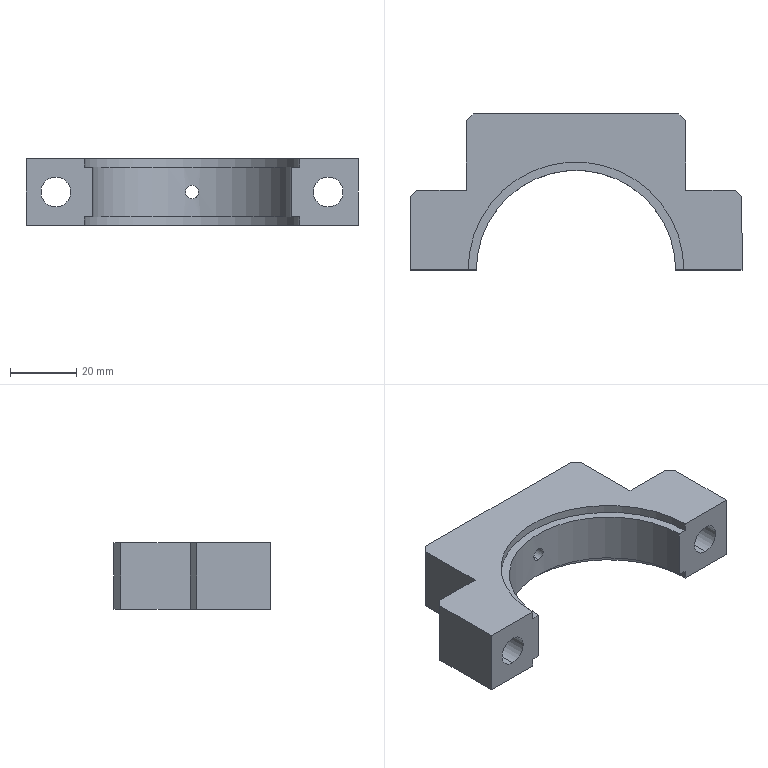Part | SolidWorks | features HoleWzd 3, ICE 2, Chamfer 1, Extrusion 1 | 1 solid | 30 faces | box 100 x 47 x 20 mm | volume 45084 mm3 | plane 17 | cylinder 11 | cone 2 | commonest cylinder face diameters 9 x4 4 x2 7 x2 65 x2 60 x1
STEP:
#1=CARTESIAN_POINT('',(0.,30.,8.));
#2=VERTEX_POINT('',#1);
#3=CARTESIAN_POINT('',(0.,30.,12.));
#4=VERTEX_POINT('',#3);
#5=CARTESIAN_POINT('',(0.,30.,8.));
#6=CARTESIAN_POINT('',(-0.261,30.,8.));
#7=CARTESIAN_POINT('',(-0.5242,29.996,8.052));
#8=CARTESIAN_POINT('',(-1.006,29.984,8.252));
#9=CARTESIAN_POINT('',(-1.229,29.975,8.401));
#10=CARTESIAN_POINT('',(-1.505,29.962,8.677));
#11=CARTESIAN_POINT('',(-1.59,29.958,8.78));
#12=CARTESIAN_POINT('',(-1.735,29.95,8.997));
#13=CARTESIAN_POINT('',(-1.797,29.946,9.112));
#14=CARTESIAN_POINT('',(-1.897,29.94,9.354));
#15=CARTESIAN_POINT('',(-1.936,29.937,9.481));
#16=CARTESIAN_POINT('',(-1.987,29.934,9.737));
#17=CARTESIAN_POINT('',(-2.,29.933,9.866));
#18=CARTESIAN_POINT('',(-2.,29.933,10.13));
#19=CARTESIAN_POINT('',(-1.987,29.934,10.261));
#20=CARTESIAN_POINT('',(-1.937,29.937,10.516));
#21=CARTESIAN_POINT('',(-1.898,29.94,10.643));
#22=CARTESIAN_POINT('',(-1.798,29.946,10.886));
#23=CARTESIAN_POINT('',(-1.737,29.95,11.001));
#24=CARTESIAN_POINT('',(-1.592,29.958,11.218));
#25=CARTESIAN_POINT('',(-1.507,29.962,11.321));
#26=CARTESIAN_POINT('',(-1.323,29.971,11.506));
#27=CARTESIAN_POINT('',(-1.222,29.975,11.588));
#28=CARTESIAN_POINT('',(-1.004,29.983,11.735));
#29=CARTESIAN_POINT('',(-0.8877,29.987,11.797));
#30=CARTESIAN_POINT('',(-0.5269,29.996,11.947));
#31=CARTESIAN_POINT('',(-0.2643,30.,12.));
#32=CARTESIAN_POINT('',(0.,30.,12.));
#33=B_SPLINE_CURVE_WITH_KNOTS('',3,(#5,#6,#7,#8,#9,#10,#11,#12,#13,#14,#15,#16,#17,#18,#19,#20,#21,#22,#23,#24,#25,#26,#27,#28,#29,#30,#31,#32),.UNSPECIFIED.,.F.,.F.,(4,2,2,2,2,2,2,2,2,2,2,2,2,4),(0.006255,0.007036,0.007818,0.008209,0.0086,0.00899,0.009381,0.009772,0.01016,0.01055,0.01094,0.01134,0.01173,0.01251),.UNSPECIFIED.);
#34=EDGE_CURVE('',#2,#4,#33,.T.);
#35=ORIENTED_EDGE('',*,*,#34,.F.);
#36=CARTESIAN_POINT('',(0.,33.099,8.));
#37=VERTEX_POINT('',#36);
#38=CARTESIAN_POINT('',(0.,47.,8.));
#39=DIRECTION('',(0.,1.,0.));
#40=VECTOR('',#39,1000.);
#41=LINE('',#38,#40);
#42=EDGE_CURVE('',#2,#37,#41,.T.);
#43=ORIENTED_EDGE('',*,*,#42,.T.);
#44=CARTESIAN_POINT('',(0.,33.099,12.));
#45=VERTEX_POINT('',#44);
#46=CARTESIAN_POINT('',(0.,33.099,10.));
#47=DIRECTION('',(0.,-1.,0.));
#48=DIRECTION('',(0.,0.,1.));
#49=AXIS2_PLACEMENT_3D('',#46,#47,#48);
#50=CIRCLE('',#49,2.);
#51=EDGE_CURVE('',#45,#37,#50,.T.);
#52=ORIENTED_EDGE('',*,*,#51,.F.);
#53=CARTESIAN_POINT('',(0.,47.,12.));
#54=DIRECTION('',(0.,1.,0.));
#55=VECTOR('',#54,1000.);
#56=LINE('',#53,#55);
#57=EDGE_CURVE('',#4,#45,#56,.T.);
#58=ORIENTED_EDGE('',*,*,#57,.F.);
#59=EDGE_LOOP('',(#35,#43,#52,#58));
#60=FACE_OUTER_BOUND('',#59,.T.);
#61=CARTESIAN_POINT('',(0.,47.,10.));
#62=DIRECTION('',(0.,1.,0.));
#63=DIRECTION('',(0.,0.,1.));
#64=AXIS2_PLACEMENT_3D('',#61,#62,#63);
#65=CYLINDRICAL_SURFACE('',#64,2.);
#66=ADVANCED_FACE('',(#60),#65,.F.);
#67=CARTESIAN_POINT('',(-41.,0.,5.5));
#68=VERTEX_POINT('',#67);
#69=CARTESIAN_POINT('',(-41.,0.,14.5));
#70=VERTEX_POINT('',#69);
#71=CARTESIAN_POINT('',(-41.,0.,10.));
#72=DIRECTION('',(0.,1.,0.));
#73=DIRECTION('',(0.,0.,1.));
#74=AXIS2_PLACEMENT_3D('',#71,#72,#73);
#75=CIRCLE('',#74,4.5);
#76=EDGE_CURVE('',#68,#70,#75,.T.);
#77=ORIENTED_EDGE('',*,*,#76,.F.);
#78=CARTESIAN_POINT('',(-41.,24.,5.5));
#79=VERTEX_POINT('',#78);
#80=CARTESIAN_POINT('',(-41.,24.,5.5));
#81=DIRECTION('',(0.,1.,0.));
#82=VECTOR('',#81,1000.);
#83=LINE('',#80,#82);
#84=EDGE_CURVE('',#68,#79,#83,.T.);
#85=ORIENTED_EDGE('',*,*,#84,.T.);
#86=CARTESIAN_POINT('',(-41.,24.,14.5));
#87=VERTEX_POINT('',#86);
#88=CARTESIAN_POINT('',(-41.,24.,10.));
#89=DIRECTION('',(0.,1.,0.));
#90=DIRECTION('',(0.,0.,1.));
#91=AXIS2_PLACEMENT_3D('',#88,#89,#90);
#92=CIRCLE('',#91,4.5);
#93=EDGE_CURVE('',#79,#87,#92,.T.);
#94=ORIENTED_EDGE('',*,*,#93,.T.);
#95=CARTESIAN_POINT('',(-41.,24.,14.5));
#96=DIRECTION('',(0.,1.,0.));
#97=VECTOR('',#96,1000.);
#98=LINE('',#95,#97);
#99=EDGE_CURVE('',#70,#87,#98,.T.);
#100=ORIENTED_EDGE('',*,*,#99,.F.);
#101=EDGE_LOOP('',(#77,#85,#94,#100));
#102=FACE_OUTER_BOUND('',#101,.T.);
#103=CARTESIAN_POINT('',(-41.,24.,10.));
#104=DIRECTION('',(0.,1.,0.));
#105=DIRECTION('',(0.,0.,1.));
#106=AXIS2_PLACEMENT_3D('',#103,#104,#105);
#107=CYLINDRICAL_SURFACE('',#106,4.5);
#108=ADVANCED_FACE('',(#102),#107,.F.);
#109=CARTESIAN_POINT('',(41.,0.,5.5));
#110=VERTEX_POINT('',#109);
#111=CARTESIAN_POINT('',(41.,0.,14.5));
#112=VERTEX_POINT('',#111);
#113=CARTESIAN_POINT('',(41.,0.,10.));
#114=DIRECTION('',(0.,1.,0.));
#115=DIRECTION('',(0.,0.,1.));
#116=AXIS2_PLACEMENT_3D('',#113,#114,#115);
#117=CIRCLE('',#116,4.5);
#118=EDGE_CURVE('',#110,#112,#117,.T.);
#119=ORIENTED_EDGE('',*,*,#118,.F.);
#120=CARTESIAN_POINT('',(41.,24.,5.5));
#121=VERTEX_POINT('',#120);
#122=CARTESIAN_POINT('',(41.,24.,5.5));
#123=DIRECTION('',(0.,1.,0.));
#124=VECTOR('',#123,1000.);
#125=LINE('',#122,#124);
#126=EDGE_CURVE('',#110,#121,#125,.T.);
#127=ORIENTED_EDGE('',*,*,#126,.T.);
#128=CARTESIAN_POINT('',(41.,24.,14.5));
#129=VERTEX_POINT('',#128);
#130=CARTESIAN_POINT('',(41.,24.,10.));
#131=DIRECTION('',(0.,1.,0.));
#132=DIRECTION('',(0.,0.,1.));
#133=AXIS2_PLACEMENT_3D('',#130,#131,#132);
#134=CIRCLE('',#133,4.5);
#135=EDGE_CURVE('',#121,#129,#134,.T.);
#136=ORIENTED_EDGE('',*,*,#135,.T.);
#137=CARTESIAN_POINT('',(41.,24.,14.5));
#138=DIRECTION('',(0.,1.,0.));
#139=VECTOR('',#138,1000.);
#140=LINE('',#137,#139);
#141=EDGE_CURVE('',#112,#129,#140,.T.);
#142=ORIENTED_EDGE('',*,*,#141,.F.);
#143=EDGE_LOOP('',(#119,#127,#136,#142));
#144=FACE_OUTER_BOUND('',#143,.T.);
#145=CARTESIAN_POINT('',(41.,24.,10.));
#146=DIRECTION('',(0.,1.,0.));
#147=DIRECTION('',(0.,0.,1.));
#148=AXIS2_PLACEMENT_3D('',#145,#146,#147);
#149=CYLINDRICAL_SURFACE('',#148,4.5);
#150=ADVANCED_FACE('',(#144),#149,.F.);
#151=CARTESIAN_POINT('',(0.,34.,6.5));
#152=VERTEX_POINT('',#151);
#153=CARTESIAN_POINT('',(0.,34.,13.5));
#154=VERTEX_POINT('',#153);
#155=CARTESIAN_POINT('',(0.,34.,10.));
#156=DIRECTION('',(0.,1.,0.));
#157=DIRECTION('',(0.,0.,1.));
#158=AXIS2_PLACEMENT_3D('',#155,#156,#157);
#159=CIRCLE('',#158,3.5);
#160=EDGE_CURVE('',#152,#154,#159,.T.);
#161=ORIENTED_EDGE('',*,*,#160,.F.);
#162=CARTESIAN_POINT('',(0.,47.,6.5));
#163=VERTEX_POINT('',#162);
#164=CARTESIAN_POINT('',(0.,47.,6.5));
#165=DIRECTION('',(0.,1.,0.));
#166=VECTOR('',#165,1000.);
#167=LINE('',#164,#166);
#168=EDGE_CURVE('',#152,#163,#167,.T.);
#169=ORIENTED_EDGE('',*,*,#168,.T.);
#170=CARTESIAN_POINT('',(0.,47.,13.5));
#171=VERTEX_POINT('',#170);
#172=CARTESIAN_POINT('',(0.,47.,10.));
#173=DIRECTION('',(0.,1.,0.));
#174=DIRECTION('',(0.,0.,1.));
#175=AXIS2_PLACEMENT_3D('',#172,#173,#174);
#176=CIRCLE('',#175,3.5);
#177=EDGE_CURVE('',#163,#171,#176,.T.);
#178=ORIENTED_EDGE('',*,*,#177,.T.);
#179=CARTESIAN_POINT('',(0.,47.,13.5));
#180=DIRECTION('',(0.,1.,0.));
#181=VECTOR('',#180,1000.);
#182=LINE('',#179,#181);
#183=EDGE_CURVE('',#154,#171,#182,.T.);
#184=ORIENTED_EDGE('',*,*,#183,.F.);
#185=EDGE_LOOP('',(#161,#169,#178,#184));
#186=FACE_OUTER_BOUND('',#185,.T.);
#187=CARTESIAN_POINT('',(0.,47.,10.));
#188=DIRECTION('',(0.,1.,0.));
#189=DIRECTION('',(0.,0.,1.));
#190=AXIS2_PLACEMENT_3D('',#187,#188,#189);
#191=CYLINDRICAL_SURFACE('',#190,3.5);
#192=ADVANCED_FACE('',(#186),#191,.F.);
#193=ORIENTED_EDGE('',*,*,#51,.T.);
#194=CARTESIAN_POINT('',(0.,34.,6.5));
#195=DIRECTION('',(0.,0.515,-0.8572));
#196=VECTOR('',#195,1000.);
#197=LINE('',#194,#196);
#198=EDGE_CURVE('',#37,#152,#197,.T.);
#199=ORIENTED_EDGE('',*,*,#198,.T.);
#200=ORIENTED_EDGE('',*,*,#160,.T.);
#201=CARTESIAN_POINT('',(0.,34.,13.5));
#202=DIRECTION('',(0.,0.515,0.8572));
#203=VECTOR('',#202,1000.);
#204=LINE('',#201,#203);
#205=EDGE_CURVE('',#45,#154,#204,.T.);
#206=ORIENTED_EDGE('',*,*,#205,.F.);
#207=EDGE_LOOP('',(#193,#199,#200,#206));
#208=FACE_OUTER_BOUND('',#207,.T.);
#209=CARTESIAN_POINT('',(0.,34.,10.));
#210=DIRECTION('',(0.,1.,0.));
#211=DIRECTION('',(0.,0.,1.));
#212=AXIS2_PLACEMENT_3D('',#209,#210,#211);
#213=CONICAL_SURFACE('',#212,3.5,1.03);
#214=ADVANCED_FACE('',(#208),#213,.F.);
#215=CARTESIAN_POINT('',(0.,30.,12.));
#216=CARTESIAN_POINT('',(0.1322,30.,12.));
#217=CARTESIAN_POINT('',(0.2622,29.999,11.987));
#218=CARTESIAN_POINT('',(0.5178,29.996,11.936));
#219=CARTESIAN_POINT('',(0.6449,29.993,11.898));
#220=CARTESIAN_POINT('',(0.8871,29.987,11.797));
#221=CARTESIAN_POINT('',(1.002,29.983,11.736));
#222=CARTESIAN_POINT('',(1.219,29.975,11.591));
#223=CARTESIAN_POINT('',(1.322,29.971,11.506));
#224=CARTESIAN_POINT('',(1.599,29.958,11.229));
#225=CARTESIAN_POINT('',(1.748,29.949,11.006));
#226=CARTESIAN_POINT('',(1.947,29.937,10.525));
#227=CARTESIAN_POINT('',(2.,29.933,10.262));
#228=CARTESIAN_POINT('',(2.,29.933,9.87));
#229=CARTESIAN_POINT('',(1.987,29.934,9.738));
#230=CARTESIAN_POINT('',(1.936,29.937,9.481));
#231=CARTESIAN_POINT('',(1.898,29.94,9.356));
#232=CARTESIAN_POINT('',(1.798,29.946,9.114));
#233=CARTESIAN_POINT('',(1.735,29.95,8.997));
#234=CARTESIAN_POINT('',(1.591,29.958,8.78));
#235=CARTESIAN_POINT('',(1.508,29.962,8.679));
#236=CARTESIAN_POINT('',(1.321,29.971,8.493));
#237=CARTESIAN_POINT('',(1.22,29.975,8.41));
#238=CARTESIAN_POINT('',(1.003,29.983,8.265));
#239=CARTESIAN_POINT('',(0.8865,29.987,8.202));
#240=CARTESIAN_POINT('',(0.6442,29.993,8.102));
#241=CARTESIAN_POINT('',(0.5195,29.996,8.064));
#242=CARTESIAN_POINT('',(0.2631,29.999,8.013));
#243=CARTESIAN_POINT('',(0.1305,30.,8.));
#244=CARTESIAN_POINT('',(0.,30.,8.));
#245=B_SPLINE_CURVE_WITH_KNOTS('',3,(#215,#216,#217,#218,#219,#220,#221,#222,#223,#224,#225,#226,#227,#228,#229,#230,#231,#232,#233,#234,#235,#236,#237,#238,#239,#240,#241,#242,#243,#244),.UNSPECIFIED.,.F.,.F.,(4,2,2,2,2,2,2,2,2,2,2,2,2,2,4),(0.,0.0003909,0.0007818,0.001173,0.001564,0.002345,0.003127,0.003518,0.003909,0.0043,0.004691,0.005082,0.005473,0.005864,0.006255),.UNSPECIFIED.);
#246=EDGE_CURVE('',#4,#2,#245,.T.);
#247=ORIENTED_EDGE('',*,*,#246,.T.);
#248=ORIENTED_EDGE('',*,*,#34,.T.);
#249=EDGE_LOOP('',(#247,#248));
#250=FACE_BOUND('',#249,.T.);
#251=CARTESIAN_POINT('',(-30.,0.,17.5));
#252=VERTEX_POINT('',#251);
#253=CARTESIAN_POINT('',(30.,0.,17.5));
#254=VERTEX_POINT('',#253);
#255=CARTESIAN_POINT('',(0.,0.,17.5));
#256=DIRECTION('',(0.,0.,-1.));
#257=DIRECTION('',(1.,0.,0.));
#258=AXIS2_PLACEMENT_3D('',#255,#256,#257);
#259=CIRCLE('',#258,30.);
#260=EDGE_CURVE('',#252,#254,#259,.T.);
#261=ORIENTED_EDGE('',*,*,#260,.F.);
#262=CARTESIAN_POINT('',(-30.,0.,2.5));
#263=VERTEX_POINT('',#262);
#264=CARTESIAN_POINT('',(-30.,0.,20.));
#265=DIRECTION('',(0.,0.,-1.));
#266=VECTOR('',#265,1000.);
#267=LINE('',#264,#266);
#268=EDGE_CURVE('',#252,#263,#267,.T.);
#269=ORIENTED_EDGE('',*,*,#268,.T.);
#270=CARTESIAN_POINT('',(30.,0.,2.5));
#271=VERTEX_POINT('',#270);
#272=CARTESIAN_POINT('',(0.,0.,2.5));
#273=DIRECTION('',(0.,0.,1.));
#274=DIRECTION('',(-1.,0.,0.));
#275=AXIS2_PLACEMENT_3D('',#272,#273,#274);
#276=CIRCLE('',#275,30.);
#277=EDGE_CURVE('',#271,#263,#276,.T.);
#278=ORIENTED_EDGE('',*,*,#277,.F.);
#279=CARTESIAN_POINT('',(30.,0.,20.));
#280=DIRECTION('',(0.,0.,-1.));
#281=VECTOR('',#280,1000.);
#282=LINE('',#279,#281);
#283=EDGE_CURVE('',#254,#271,#282,.T.);
#284=ORIENTED_EDGE('',*,*,#283,.F.);
#285=EDGE_LOOP('',(#261,#269,#278,#284));
#286=FACE_OUTER_BOUND('',#285,.T.);
#287=CARTESIAN_POINT('',(0.,0.,20.));
#288=DIRECTION('',(0.,0.,-1.));
#289=DIRECTION('',(-1.,0.,0.));
#290=AXIS2_PLACEMENT_3D('',#287,#288,#289);
#291=CYLINDRICAL_SURFACE('',#290,30.);
#292=ADVANCED_FACE('',(#250,#286),#291,.F.);
#293=CARTESIAN_POINT('',(-50.,22.,20.));
#294=VERTEX_POINT('',#293);
#295=CARTESIAN_POINT('',(-50.,0.,20.));
#296=VERTEX_POINT('',#295);
#297=CARTESIAN_POINT('',(-50.,0.,20.));
#298=DIRECTION('',(0.,-1.,0.));
#299=VECTOR('',#298,1000.);
#300=LINE('',#297,#299);
#301=EDGE_CURVE('',#294,#296,#300,.T.);
#302=ORIENTED_EDGE('',*,*,#301,.F.);
#303=CARTESIAN_POINT('',(-50.,22.,0.));
#304=VERTEX_POINT('',#303);
#305=CARTESIAN_POINT('',(-50.,22.,20.));
#306=DIRECTION('',(0.,0.,-1.));
#307=VECTOR('',#306,1000.);
#308=LINE('',#305,#307);
#309=EDGE_CURVE('',#294,#304,#308,.T.);
#310=ORIENTED_EDGE('',*,*,#309,.T.);
#311=CARTESIAN_POINT('',(-50.,0.,0.));
#312=VERTEX_POINT('',#311);
#313=CARTESIAN_POINT('',(-50.,0.,0.));
#314=DIRECTION('',(0.,-1.,0.));
#315=VECTOR('',#314,1000.);
#316=LINE('',#313,#315);
#317=EDGE_CURVE('',#304,#312,#316,.T.);
#318=ORIENTED_EDGE('',*,*,#317,.T.);
#319=CARTESIAN_POINT('',(-50.,0.,20.));
#320=DIRECTION('',(0.,0.,-1.));
#321=VECTOR('',#320,1000.);
#322=LINE('',#319,#321);
#323=EDGE_CURVE('',#296,#312,#322,.T.);
#324=ORIENTED_EDGE('',*,*,#323,.F.);
#325=EDGE_LOOP('',(#302,#310,#318,#324));
#326=FACE_OUTER_BOUND('',#325,.T.);
#327=CARTESIAN_POINT('',(-50.,0.,20.));
#328=DIRECTION('',(1.,0.,0.));
#329=DIRECTION('',(0.,0.,-1.));
#330=AXIS2_PLACEMENT_3D('',#327,#328,#329);
#331=PLANE('',#330);
#332=ADVANCED_FACE('',(#326),#331,.F.);
#333=CARTESIAN_POINT('',(-41.,0.,10.));
#334=DIRECTION('',(0.,1.,0.));
#335=DIRECTION('',(0.,0.,1.));
#336=AXIS2_PLACEMENT_3D('',#333,#334,#335);
#337=CIRCLE('',#336,4.5);
#338=EDGE_CURVE('',#70,#68,#337,.T.);
#339=ORIENTED_EDGE('',*,*,#338,.T.);
#340=ORIENTED_EDGE('',*,*,#76,.T.);
#341=EDGE_LOOP('',(#339,#340));
#342=FACE_BOUND('',#341,.T.);
#343=CARTESIAN_POINT('',(-32.5,0.,17.5));
#344=VERTEX_POINT('',#343);
#345=CARTESIAN_POINT('',(-50.,0.,17.5));
#346=DIRECTION('',(1.,0.,0.));
#347=VECTOR('',#346,1000.);
#348=LINE('',#345,#347);
#349=EDGE_CURVE('',#344,#252,#348,.T.);
#350=ORIENTED_EDGE('',*,*,#349,.F.);
#351=CARTESIAN_POINT('',(-32.5,0.,20.));
#352=VERTEX_POINT('',#351);
#353=CARTESIAN_POINT('',(-32.5,0.,17.5));
#354=DIRECTION('',(0.,0.,1.));
#355=VECTOR('',#354,1000.);
#356=LINE('',#353,#355);
#357=EDGE_CURVE('',#344,#352,#356,.T.);
#358=ORIENTED_EDGE('',*,*,#357,.T.);
#359=CARTESIAN_POINT('',(-50.,0.,20.));
#360=DIRECTION('',(1.,0.,0.));
#361=VECTOR('',#360,1000.);
#362=LINE('',#359,#361);
#363=EDGE_CURVE('',#296,#352,#362,.T.);
#364=ORIENTED_EDGE('',*,*,#363,.F.);
#365=ORIENTED_EDGE('',*,*,#323,.T.);
#366=CARTESIAN_POINT('',(-32.5,0.,0.));
#367=VERTEX_POINT('',#366);
#368=CARTESIAN_POINT('',(-50.,0.,0.));
#369=DIRECTION('',(1.,0.,0.));
#370=VECTOR('',#369,1000.);
#371=LINE('',#368,#370);
#372=EDGE_CURVE('',#312,#367,#371,.T.);
#373=ORIENTED_EDGE('',*,*,#372,.T.);
#374=CARTESIAN_POINT('',(-32.5,0.,2.5));
#375=VERTEX_POINT('',#374);
#376=CARTESIAN_POINT('',(-32.5,0.,2.5));
#377=DIRECTION('',(0.,0.,1.));
#378=VECTOR('',#377,1000.);
#379=LINE('',#376,#378);
#380=EDGE_CURVE('',#367,#375,#379,.T.);
#381=ORIENTED_EDGE('',*,*,#380,.T.);
#382=CARTESIAN_POINT('',(-50.,0.,2.5));
#383=DIRECTION('',(-1.,0.,0.));
#384=VECTOR('',#383,1000.);
#385=LINE('',#382,#384);
#386=EDGE_CURVE('',#263,#375,#385,.T.);
#387=ORIENTED_EDGE('',*,*,#386,.F.);
#388=ORIENTED_EDGE('',*,*,#268,.F.);
#389=EDGE_LOOP('',(#350,#358,#364,#365,#373,#381,#387,#388));
#390=FACE_OUTER_BOUND('',#389,.T.);
#391=CARTESIAN_POINT('',(-50.,0.,20.));
#392=DIRECTION('',(0.,1.,0.));
#393=DIRECTION('',(-1.,0.,0.));
#394=AXIS2_PLACEMENT_3D('',#391,#392,#393);
#395=PLANE('',#394);
#396=ADVANCED_FACE('',(#342,#390),#395,.F.);
#397=CARTESIAN_POINT('',(41.,0.,10.));
#398=DIRECTION('',(0.,1.,0.));
#399=DIRECTION('',(0.,0.,1.));
#400=AXIS2_PLACEMENT_3D('',#397,#398,#399);
#401=CIRCLE('',#400,4.5);
#402=EDGE_CURVE('',#112,#110,#401,.T.);
#403=ORIENTED_EDGE('',*,*,#402,.T.);
#404=ORIENTED_EDGE('',*,*,#118,.T.);
#405=EDGE_LOOP('',(#403,#404));
#406=FACE_BOUND('',#405,.T.);
#407=CARTESIAN_POINT('',(32.5,0.,20.));
#408=VERTEX_POINT('',#407);
#409=CARTESIAN_POINT('',(50.,0.,20.));
#410=VERTEX_POINT('',#409);
#411=CARTESIAN_POINT('',(30.,0.,20.));
#412=DIRECTION('',(1.,0.,0.));
#413=VECTOR('',#412,1000.);
#414=LINE('',#411,#413);
#415=EDGE_CURVE('',#408,#410,#414,.T.);
#416=ORIENTED_EDGE('',*,*,#415,.F.);
#417=CARTESIAN_POINT('',(32.5,0.,17.5));
#418=VERTEX_POINT('',#417);
#419=CARTESIAN_POINT('',(32.5,0.,17.5));
#420=DIRECTION('',(0.,0.,-1.));
#421=VECTOR('',#420,1000.);
#422=LINE('',#419,#421);
#423=EDGE_CURVE('',#408,#418,#422,.T.);
#424=ORIENTED_EDGE('',*,*,#423,.T.);
#425=CARTESIAN_POINT('',(30.,0.,17.5));
#426=DIRECTION('',(1.,0.,0.));
#427=VECTOR('',#426,1000.);
#428=LINE('',#425,#427);
#429=EDGE_CURVE('',#254,#418,#428,.T.);
#430=ORIENTED_EDGE('',*,*,#429,.F.);
#431=ORIENTED_EDGE('',*,*,#283,.T.);
#432=CARTESIAN_POINT('',(32.5,0.,2.5));
#433=VERTEX_POINT('',#432);
#434=CARTESIAN_POINT('',(30.,0.,2.5));
#435=DIRECTION('',(-1.,0.,0.));
#436=VECTOR('',#435,1000.);
#437=LINE('',#434,#436);
#438=EDGE_CURVE('',#433,#271,#437,.T.);
#439=ORIENTED_EDGE('',*,*,#438,.F.);
#440=CARTESIAN_POINT('',(32.5,0.,0.));
#441=VERTEX_POINT('',#440);
#442=CARTESIAN_POINT('',(32.5,0.,2.5));
#443=DIRECTION('',(0.,0.,-1.));
#444=VECTOR('',#443,1000.);
#445=LINE('',#442,#444);
#446=EDGE_CURVE('',#433,#441,#445,.T.);
#447=ORIENTED_EDGE('',*,*,#446,.T.);
#448=CARTESIAN_POINT('',(50.,0.,0.));
#449=VERTEX_POINT('',#448);
#450=CARTESIAN_POINT('',(30.,0.,0.));
#451=DIRECTION('',(1.,0.,0.));
#452=VECTOR('',#451,1000.);
#453=LINE('',#450,#452);
#454=EDGE_CURVE('',#441,#449,#453,.T.);
#455=ORIENTED_EDGE('',*,*,#454,.T.);
#456=CARTESIAN_POINT('',(50.,0.,20.));
#457=DIRECTION('',(0.,0.,-1.));
#458=VECTOR('',#457,1000.);
#459=LINE('',#456,#458);
#460=EDGE_CURVE('',#410,#449,#459,.T.);
#461=ORIENTED_EDGE('',*,*,#460,.F.);
#462=EDGE_LOOP('',(#416,#424,#430,#431,#439,#447,#455,#461));
#463=FACE_OUTER_BOUND('',#462,.T.);
#464=CARTESIAN_POINT('',(30.,0.,20.));
#465=DIRECTION('',(0.,1.,0.));
#466=DIRECTION('',(-1.,0.,0.));
#467=AXIS2_PLACEMENT_3D('',#464,#465,#466);
#468=PLANE('',#467);
#469=ADVANCED_FACE('',(#406,#463),#468,.F.);
#470=CARTESIAN_POINT('',(50.,22.,0.));
#471=VERTEX_POINT('',#470);
#472=CARTESIAN_POINT('',(50.,0.,0.));
#473=DIRECTION('',(0.,1.,0.));
#474=VECTOR('',#473,1000.);
#475=LINE('',#472,#474);
#476=EDGE_CURVE('',#449,#471,#475,.T.);
#477=ORIENTED_EDGE('',*,*,#476,.T.);
#478=CARTESIAN_POINT('',(50.,22.,20.));
#479=VERTEX_POINT('',#478);
#480=CARTESIAN_POINT('',(50.,22.,20.));
#481=DIRECTION('',(0.,0.,1.));
#482=VECTOR('',#481,1000.);
#483=LINE('',#480,#482);
#484=EDGE_CURVE('',#471,#479,#483,.T.);
#485=ORIENTED_EDGE('',*,*,#484,.T.);
#486=CARTESIAN_POINT('',(50.,0.,20.));
#487=DIRECTION('',(0.,1.,0.));
#488=VECTOR('',#487,1000.);
#489=LINE('',#486,#488);
#490=EDGE_CURVE('',#410,#479,#489,.T.);
#491=ORIENTED_EDGE('',*,*,#490,.F.);
#492=ORIENTED_EDGE('',*,*,#460,.T.);
#493=EDGE_LOOP('',(#477,#485,#491,#492));
#494=FACE_OUTER_BOUND('',#493,.T.);
#495=CARTESIAN_POINT('',(50.,0.,20.));
#496=DIRECTION('',(-1.,0.,0.));
#497=DIRECTION('',(0.,-1.,0.));
#498=AXIS2_PLACEMENT_3D('',#495,#496,#497);
#499=PLANE('',#498);
#500=ADVANCED_FACE('',(#494),#499,.F.);
#501=CARTESIAN_POINT('',(41.,24.,10.));
#502=DIRECTION('',(0.,1.,0.));
#503=DIRECTION('',(0.,0.,1.));
#504=AXIS2_PLACEMENT_3D('',#501,#502,#503);
#505=CIRCLE('',#504,4.5);
#506=EDGE_CURVE('',#129,#121,#505,.T.);
#507=ORIENTED_EDGE('',*,*,#506,.F.);
#508=ORIENTED_EDGE('',*,*,#135,.F.);
#509=EDGE_LOOP('',(#507,#508));
#510=FACE_BOUND('',#509,.T.);
#511=CARTESIAN_POINT('',(48.,24.,20.));
#512=VERTEX_POINT('',#511);
#513=CARTESIAN_POINT('',(33.,24.,20.));
#514=VERTEX_POINT('',#513);
#515=CARTESIAN_POINT('',(50.,24.,20.));
#516=DIRECTION('',(-1.,0.,0.));
#517=VECTOR('',#516,1000.);
#518=LINE('',#515,#517);
#519=EDGE_CURVE('',#512,#514,#518,.T.);
#520=ORIENTED_EDGE('',*,*,#519,.F.);
#521=CARTESIAN_POINT('',(48.,24.,0.));
#522=VERTEX_POINT('',#521);
#523=CARTESIAN_POINT('',(48.,24.,20.));
#524=DIRECTION('',(0.,0.,-1.));
#525=VECTOR('',#524,1000.);
#526=LINE('',#523,#525);
#527=EDGE_CURVE('',#512,#522,#526,.T.);
#528=ORIENTED_EDGE('',*,*,#527,.T.);
#529=CARTESIAN_POINT('',(33.,24.,0.));
#530=VERTEX_POINT('',#529);
#531=CARTESIAN_POINT('',(50.,24.,0.));
#532=DIRECTION('',(-1.,0.,0.));
#533=VECTOR('',#532,1000.);
#534=LINE('',#531,#533);
#535=EDGE_CURVE('',#522,#530,#534,.T.);
#536=ORIENTED_EDGE('',*,*,#535,.T.);
#537=CARTESIAN_POINT('',(33.,24.,20.));
#538=DIRECTION('',(0.,0.,-1.));
#539=VECTOR('',#538,1000.);
#540=LINE('',#537,#539);
#541=EDGE_CURVE('',#514,#530,#540,.T.);
#542=ORIENTED_EDGE('',*,*,#541,.F.);
#543=EDGE_LOOP('',(#520,#528,#536,#542));
#544=FACE_OUTER_BOUND('',#543,.T.);
#545=CARTESIAN_POINT('',(50.,24.,20.));
#546=DIRECTION('',(0.,-1.,0.));
#547=DIRECTION('',(1.,0.,0.));
#548=AXIS2_PLACEMENT_3D('',#545,#546,#547);
#549=PLANE('',#548);
#550=ADVANCED_FACE('',(#510,#544),#549,.F.);
#551=CARTESIAN_POINT('',(33.,45.,0.));
#552=VERTEX_POINT('',#551);
#553=CARTESIAN_POINT('',(33.,24.,0.));
#554=DIRECTION('',(0.,1.,0.));
#555=VECTOR('',#554,1000.);
#556=LINE('',#553,#555);
#557=EDGE_CURVE('',#530,#552,#556,.T.);
#558=ORIENTED_EDGE('',*,*,#557,.T.);
#559=CARTESIAN_POINT('',(33.,45.,20.));
#560=VERTEX_POINT('',#559);
#561=CARTESIAN_POINT('',(33.,45.,20.));
#562=DIRECTION('',(0.,0.,1.));
#563=VECTOR('',#562,1000.);
#564=LINE('',#561,#563);
#565=EDGE_CURVE('',#552,#560,#564,.T.);
#566=ORIENTED_EDGE('',*,*,#565,.T.);
#567=CARTESIAN_POINT('',(33.,24.,20.));
#568=DIRECTION('',(0.,1.,0.));
#569=VECTOR('',#568,1000.);
#570=LINE('',#567,#569);
#571=EDGE_CURVE('',#514,#560,#570,.T.);
#572=ORIENTED_EDGE('',*,*,#571,.F.);
#573=ORIENTED_EDGE('',*,*,#541,.T.);
#574=EDGE_LOOP('',(#558,#566,#572,#573));
#575=FACE_OUTER_BOUND('',#574,.T.);
#576=CARTESIAN_POINT('',(33.,24.,20.));
#577=DIRECTION('',(-1.,0.,0.));
#578=DIRECTION('',(0.,-1.,0.));
#579=AXIS2_PLACEMENT_3D('',#576,#577,#578);
#580=PLANE('',#579);
#581=ADVANCED_FACE('',(#575),#580,.F.);
#582=CARTESIAN_POINT('',(0.,47.,10.));
#583=DIRECTION('',(0.,1.,0.));
#584=DIRECTION('',(0.,0.,1.));
#585=AXIS2_PLACEMENT_3D('',#582,#583,#584);
#586=CIRCLE('',#585,3.5);
#587=EDGE_CURVE('',#171,#163,#586,.T.);
#588=ORIENTED_EDGE('',*,*,#587,.F.);
#589=ORIENTED_EDGE('',*,*,#177,.F.);
#590=EDGE_LOOP('',(#588,#589));
#591=FACE_BOUND('',#590,.T.);
#592=CARTESIAN_POINT('',(31.,47.,20.));
#593=VERTEX_POINT('',#592);
#594=CARTESIAN_POINT('',(-31.,47.,20.));
#595=VERTEX_POINT('',#594);
#596=CARTESIAN_POINT('',(-33.,47.,20.));
#597=DIRECTION('',(-1.,0.,0.));
#598=VECTOR('',#597,1000.);
#599=LINE('',#596,#598);
#600=EDGE_CURVE('',#593,#595,#599,.T.);
#601=ORIENTED_EDGE('',*,*,#600,.F.);
#602=CARTESIAN_POINT('',(31.,47.,0.));
#603=VERTEX_POINT('',#602);
#604=CARTESIAN_POINT('',(31.,47.,20.));
#605=DIRECTION('',(0.,0.,-1.));
#606=VECTOR('',#605,1000.);
#607=LINE('',#604,#606);
#608=EDGE_CURVE('',#593,#603,#607,.T.);
#609=ORIENTED_EDGE('',*,*,#608,.T.);
#610=CARTESIAN_POINT('',(-31.,47.,0.));
#611=VERTEX_POINT('',#610);
#612=CARTESIAN_POINT('',(-33.,47.,0.));
#613=DIRECTION('',(-1.,0.,0.));
#614=VECTOR('',#613,1000.);
#615=LINE('',#612,#614);
#616=EDGE_CURVE('',#603,#611,#615,.T.);
#617=ORIENTED_EDGE('',*,*,#616,.T.);
#618=CARTESIAN_POINT('',(-31.,47.,20.));
#619=DIRECTION('',(0.,0.,1.));
#620=VECTOR('',#619,1000.);
#621=LINE('',#618,#620);
#622=EDGE_CURVE('',#611,#595,#621,.T.);
#623=ORIENTED_EDGE('',*,*,#622,.T.);
#624=EDGE_LOOP('',(#601,#609,#617,#623));
#625=FACE_OUTER_BOUND('',#624,.T.);
#626=CARTESIAN_POINT('',(-33.,47.,20.));
#627=DIRECTION('',(0.,-1.,0.));
#628=DIRECTION('',(1.,0.,0.));
#629=AXIS2_PLACEMENT_3D('',#626,#627,#628);
#630=PLANE('',#629);
#631=ADVANCED_FACE('',(#591,#625),#630,.F.);
#632=CARTESIAN_POINT('',(-33.,45.,20.));
#633=VERTEX_POINT('',#632);
#634=CARTESIAN_POINT('',(-33.,24.,20.));
#635=VERTEX_POINT('',#634);
#636=CARTESIAN_POINT('',(-33.,24.,20.));
#637=DIRECTION('',(0.,-1.,0.));
#638=VECTOR('',#637,1000.);
#639=LINE('',#636,#638);
#640=EDGE_CURVE('',#633,#635,#639,.T.);
#641=ORIENTED_EDGE('',*,*,#640,.F.);
#642=CARTESIAN_POINT('',(-33.,45.,0.));
#643=VERTEX_POINT('',#642);
#644=CARTESIAN_POINT('',(-33.,45.,20.));
#645=DIRECTION('',(0.,0.,-1.));
#646=VECTOR('',#645,1000.);
#647=LINE('',#644,#646);
#648=EDGE_CURVE('',#633,#643,#647,.T.);
#649=ORIENTED_EDGE('',*,*,#648,.T.);
#650=CARTESIAN_POINT('',(-33.,24.,0.));
#651=VERTEX_POINT('',#650);
#652=CARTESIAN_POINT('',(-33.,24.,0.));
#653=DIRECTION('',(0.,-1.,0.));
#654=VECTOR('',#653,1000.);
#655=LINE('',#652,#654);
#656=EDGE_CURVE('',#643,#651,#655,.T.);
#657=ORIENTED_EDGE('',*,*,#656,.T.);
#658=CARTESIAN_POINT('',(-33.,24.,20.));
#659=DIRECTION('',(0.,0.,-1.));
#660=VECTOR('',#659,1000.);
#661=LINE('',#658,#660);
#662=EDGE_CURVE('',#635,#651,#661,.T.);
#663=ORIENTED_EDGE('',*,*,#662,.F.);
#664=EDGE_LOOP('',(#641,#649,#657,#663));
#665=FACE_OUTER_BOUND('',#664,.T.);
#666=CARTESIAN_POINT('',(-33.,24.,20.));
#667=DIRECTION('',(1.,0.,0.));
#668=DIRECTION('',(0.,1.,0.));
#669=AXIS2_PLACEMENT_3D('',#666,#667,#668);
#670=PLANE('',#669);
#671=ADVANCED_FACE('',(#665),#670,.F.);
#672=CARTESIAN_POINT('',(-41.,24.,10.));
#673=DIRECTION('',(0.,1.,0.));
#674=DIRECTION('',(0.,0.,1.));
#675=AXIS2_PLACEMENT_3D('',#672,#673,#674);
#676=CIRCLE('',#675,4.5);
#677=EDGE_CURVE('',#87,#79,#676,.T.);
#678=ORIENTED_EDGE('',*,*,#677,.F.);
#679=ORIENTED_EDGE('',*,*,#93,.F.);
#680=EDGE_LOOP('',(#678,#679));
#681=FACE_BOUND('',#680,.T.);
#682=CARTESIAN_POINT('',(-48.,24.,0.));
#683=VERTEX_POINT('',#682);
#684=CARTESIAN_POINT('',(-50.,24.,0.));
#685=DIRECTION('',(-1.,0.,0.));
#686=VECTOR('',#685,1000.);
#687=LINE('',#684,#686);
#688=EDGE_CURVE('',#651,#683,#687,.T.);
#689=ORIENTED_EDGE('',*,*,#688,.T.);
#690=CARTESIAN_POINT('',(-48.,24.,20.));
#691=VERTEX_POINT('',#690);
#692=CARTESIAN_POINT('',(-48.,24.,20.));
#693=DIRECTION('',(0.,0.,1.));
#694=VECTOR('',#693,1000.);
#695=LINE('',#692,#694);
#696=EDGE_CURVE('',#683,#691,#695,.T.);
#697=ORIENTED_EDGE('',*,*,#696,.T.);
#698=CARTESIAN_POINT('',(-50.,24.,20.));
#699=DIRECTION('',(-1.,0.,0.));
#700=VECTOR('',#699,1000.);
#701=LINE('',#698,#700);
#702=EDGE_CURVE('',#635,#691,#701,.T.);
#703=ORIENTED_EDGE('',*,*,#702,.F.);
#704=ORIENTED_EDGE('',*,*,#662,.T.);
#705=EDGE_LOOP('',(#689,#697,#703,#704));
#706=FACE_OUTER_BOUND('',#705,.T.);
#707=CARTESIAN_POINT('',(-50.,24.,20.));
#708=DIRECTION('',(0.,-1.,0.));
#709=DIRECTION('',(1.,0.,0.));
#710=AXIS2_PLACEMENT_3D('',#707,#708,#709);
#711=PLANE('',#710);
#712=ADVANCED_FACE('',(#681,#706),#711,.F.);
#713=CARTESIAN_POINT('',(0.,0.,20.));
#714=DIRECTION('',(0.,0.,1.));
#715=DIRECTION('',(1.,0.,0.));
#716=AXIS2_PLACEMENT_3D('',#713,#714,#715);
#717=CIRCLE('',#716,32.5);
#718=EDGE_CURVE('',#408,#352,#717,.T.);
#719=ORIENTED_EDGE('',*,*,#718,.F.);
#720=ORIENTED_EDGE('',*,*,#415,.T.);
#721=ORIENTED_EDGE('',*,*,#490,.T.);
#722=CARTESIAN_POINT('',(36.,36.,20.));
#723=DIRECTION('',(-0.7071,0.7071,0.));
#724=VECTOR('',#723,1000.);
#725=LINE('',#722,#724);
#726=EDGE_CURVE('',#479,#512,#725,.T.);
#727=ORIENTED_EDGE('',*,*,#726,.T.);
#728=ORIENTED_EDGE('',*,*,#519,.T.);
#729=ORIENTED_EDGE('',*,*,#571,.T.);
#730=CARTESIAN_POINT('',(39.,39.,20.));
#731=DIRECTION('',(-0.7071,0.7071,0.));
#732=VECTOR('',#731,1000.);
#733=LINE('',#730,#732);
#734=EDGE_CURVE('',#560,#593,#733,.T.);
#735=ORIENTED_EDGE('',*,*,#734,.T.);
#736=ORIENTED_EDGE('',*,*,#600,.T.);
#737=CARTESIAN_POINT('',(-39.,39.,20.));
#738=DIRECTION('',(-0.7071,-0.7071,0.));
#739=VECTOR('',#738,1000.);
#740=LINE('',#737,#739);
#741=EDGE_CURVE('',#595,#633,#740,.T.);
#742=ORIENTED_EDGE('',*,*,#741,.T.);
#743=ORIENTED_EDGE('',*,*,#640,.T.);
#744=ORIENTED_EDGE('',*,*,#702,.T.);
#745=CARTESIAN_POINT('',(-36.,36.,20.));
#746=DIRECTION('',(-0.7071,-0.7071,0.));
#747=VECTOR('',#746,1000.);
#748=LINE('',#745,#747);
#749=EDGE_CURVE('',#691,#294,#748,.T.);
#750=ORIENTED_EDGE('',*,*,#749,.T.);
#751=ORIENTED_EDGE('',*,*,#301,.T.);
#752=ORIENTED_EDGE('',*,*,#363,.T.);
#753=EDGE_LOOP('',(#719,#720,#721,#727,#728,#729,#735,#736,#742,#743,#744,#750,#751,#752));
#754=FACE_OUTER_BOUND('',#753,.T.);
#755=CARTESIAN_POINT('',(0.,0.,20.));
#756=DIRECTION('',(0.,0.,1.));
#757=DIRECTION('',(1.,0.,0.));
#758=AXIS2_PLACEMENT_3D('',#755,#756,#757);
#759=PLANE('',#758);
#760=ADVANCED_FACE('',(#754),#759,.T.);
#761=ORIENTED_EDGE('',*,*,#454,.F.);
#762=CARTESIAN_POINT('',(0.,0.,0.));
#763=DIRECTION('',(0.,0.,-1.));
#764=DIRECTION('',(-1.,0.,0.));
#765=AXIS2_PLACEMENT_3D('',#762,#763,#764);
#766=CIRCLE('',#765,32.5);
#767=EDGE_CURVE('',#367,#441,#766,.T.);
#768=ORIENTED_EDGE('',*,*,#767,.F.);
#769=ORIENTED_EDGE('',*,*,#372,.F.);
#770=ORIENTED_EDGE('',*,*,#317,.F.);
#771=CARTESIAN_POINT('',(-50.,22.,0.));
#772=DIRECTION('',(0.7071,0.7071,0.));
#773=VECTOR('',#772,1000.);
#774=LINE('',#771,#773);
#775=EDGE_CURVE('',#304,#683,#774,.T.);
#776=ORIENTED_EDGE('',*,*,#775,.T.);
#777=ORIENTED_EDGE('',*,*,#688,.F.);
#778=ORIENTED_EDGE('',*,*,#656,.F.);
#779=CARTESIAN_POINT('',(-33.,45.,0.));
#780=DIRECTION('',(0.7071,0.7071,0.));
#781=VECTOR('',#780,1000.);
#782=LINE('',#779,#781);
#783=EDGE_CURVE('',#643,#611,#782,.T.);
#784=ORIENTED_EDGE('',*,*,#783,.T.);
#785=ORIENTED_EDGE('',*,*,#616,.F.);
#786=CARTESIAN_POINT('',(31.,47.,0.));
#787=DIRECTION('',(0.7071,-0.7071,0.));
#788=VECTOR('',#787,1000.);
#789=LINE('',#786,#788);
#790=EDGE_CURVE('',#603,#552,#789,.T.);
#791=ORIENTED_EDGE('',*,*,#790,.T.);
#792=ORIENTED_EDGE('',*,*,#557,.F.);
#793=ORIENTED_EDGE('',*,*,#535,.F.);
#794=CARTESIAN_POINT('',(48.,24.,0.));
#795=DIRECTION('',(0.7071,-0.7071,0.));
#796=VECTOR('',#795,1000.);
#797=LINE('',#794,#796);
#798=EDGE_CURVE('',#522,#471,#797,.T.);
#799=ORIENTED_EDGE('',*,*,#798,.T.);
#800=ORIENTED_EDGE('',*,*,#476,.F.);
#801=EDGE_LOOP('',(#761,#768,#769,#770,#776,#777,#778,#784,#785,#791,#792,#793,#799,#800));
#802=FACE_OUTER_BOUND('',#801,.T.);
#803=CARTESIAN_POINT('',(0.,0.,0.));
#804=DIRECTION('',(0.,0.,1.));
#805=DIRECTION('',(1.,0.,0.));
#806=AXIS2_PLACEMENT_3D('',#803,#804,#805);
#807=PLANE('',#806);
#808=ADVANCED_FACE('',(#802),#807,.F.);
#809=ORIENTED_EDGE('',*,*,#726,.F.);
#810=ORIENTED_EDGE('',*,*,#484,.F.);
#811=ORIENTED_EDGE('',*,*,#798,.F.);
#812=ORIENTED_EDGE('',*,*,#527,.F.);
#813=EDGE_LOOP('',(#809,#810,#811,#812));
#814=FACE_OUTER_BOUND('',#813,.T.);
#815=CARTESIAN_POINT('',(48.,24.,20.));
#816=DIRECTION('',(-0.7071,-0.7071,0.));
#817=DIRECTION('',(0.,0.,-1.));
#818=AXIS2_PLACEMENT_3D('',#815,#816,#817);
#819=PLANE('',#818);
#820=ADVANCED_FACE('',(#814),#819,.F.);
#821=ORIENTED_EDGE('',*,*,#734,.F.);
#822=ORIENTED_EDGE('',*,*,#565,.F.);
#823=ORIENTED_EDGE('',*,*,#790,.F.);
#824=ORIENTED_EDGE('',*,*,#608,.F.);
#825=EDGE_LOOP('',(#821,#822,#823,#824));
#826=FACE_OUTER_BOUND('',#825,.T.);
#827=CARTESIAN_POINT('',(31.,47.,20.));
#828=DIRECTION('',(-0.7071,-0.7071,0.));
#829=DIRECTION('',(0.,0.,-1.));
#830=AXIS2_PLACEMENT_3D('',#827,#828,#829);
#831=PLANE('',#830);
#832=ADVANCED_FACE('',(#826),#831,.F.);
#833=ORIENTED_EDGE('',*,*,#741,.F.);
#834=ORIENTED_EDGE('',*,*,#622,.F.);
#835=ORIENTED_EDGE('',*,*,#783,.F.);
#836=ORIENTED_EDGE('',*,*,#648,.F.);
#837=EDGE_LOOP('',(#833,#834,#835,#836));
#838=FACE_OUTER_BOUND('',#837,.T.);
#839=CARTESIAN_POINT('',(-33.,45.,20.));
#840=DIRECTION('',(0.7071,-0.7071,0.));
#841=DIRECTION('',(0.,0.,-1.));
#842=AXIS2_PLACEMENT_3D('',#839,#840,#841);
#843=PLANE('',#842);
#844=ADVANCED_FACE('',(#838),#843,.F.);
#845=ORIENTED_EDGE('',*,*,#749,.F.);
#846=ORIENTED_EDGE('',*,*,#696,.F.);
#847=ORIENTED_EDGE('',*,*,#775,.F.);
#848=ORIENTED_EDGE('',*,*,#309,.F.);
#849=EDGE_LOOP('',(#845,#846,#847,#848));
#850=FACE_OUTER_BOUND('',#849,.T.);
#851=CARTESIAN_POINT('',(-50.,22.,20.));
#852=DIRECTION('',(0.7071,-0.7071,0.));
#853=DIRECTION('',(0.,0.,-1.));
#854=AXIS2_PLACEMENT_3D('',#851,#852,#853);
#855=PLANE('',#854);
#856=ADVANCED_FACE('',(#850),#855,.F.);
#857=ORIENTED_EDGE('',*,*,#198,.F.);
#858=CARTESIAN_POINT('',(0.,33.099,10.));
#859=DIRECTION('',(0.,-1.,0.));
#860=DIRECTION('',(0.,0.,1.));
#861=AXIS2_PLACEMENT_3D('',#858,#859,#860);
#862=CIRCLE('',#861,2.);
#863=EDGE_CURVE('',#37,#45,#862,.T.);
#864=ORIENTED_EDGE('',*,*,#863,.T.);
#865=ORIENTED_EDGE('',*,*,#205,.T.);
#866=CARTESIAN_POINT('',(0.,34.,10.));
#867=DIRECTION('',(0.,1.,0.));
#868=DIRECTION('',(0.,0.,1.));
#869=AXIS2_PLACEMENT_3D('',#866,#867,#868);
#870=CIRCLE('',#869,3.5);
#871=EDGE_CURVE('',#154,#152,#870,.T.);
#872=ORIENTED_EDGE('',*,*,#871,.T.);
#873=EDGE_LOOP('',(#857,#864,#865,#872));
#874=FACE_OUTER_BOUND('',#873,.T.);
#875=CARTESIAN_POINT('',(0.,34.,10.));
#876=DIRECTION('',(0.,1.,0.));
#877=DIRECTION('',(0.,0.,1.));
#878=AXIS2_PLACEMENT_3D('',#875,#876,#877);
#879=CONICAL_SURFACE('',#878,3.5,1.03);
#880=ADVANCED_FACE('',(#874),#879,.F.);
#881=ORIENTED_EDGE('',*,*,#168,.F.);
#882=ORIENTED_EDGE('',*,*,#871,.F.);
#883=ORIENTED_EDGE('',*,*,#183,.T.);
#884=ORIENTED_EDGE('',*,*,#587,.T.);
#885=EDGE_LOOP('',(#881,#882,#883,#884));
#886=FACE_OUTER_BOUND('',#885,.T.);
#887=CARTESIAN_POINT('',(0.,47.,10.));
#888=DIRECTION('',(0.,1.,0.));
#889=DIRECTION('',(0.,0.,1.));
#890=AXIS2_PLACEMENT_3D('',#887,#888,#889);
#891=CYLINDRICAL_SURFACE('',#890,3.5);
#892=ADVANCED_FACE('',(#886),#891,.F.);
#893=ORIENTED_EDGE('',*,*,#126,.F.);
#894=ORIENTED_EDGE('',*,*,#402,.F.);
#895=ORIENTED_EDGE('',*,*,#141,.T.);
#896=ORIENTED_EDGE('',*,*,#506,.T.);
#897=EDGE_LOOP('',(#893,#894,#895,#896));
#898=FACE_OUTER_BOUND('',#897,.T.);
#899=CARTESIAN_POINT('',(41.,24.,10.));
#900=DIRECTION('',(0.,1.,0.));
#901=DIRECTION('',(0.,0.,1.));
#902=AXIS2_PLACEMENT_3D('',#899,#900,#901);
#903=CYLINDRICAL_SURFACE('',#902,4.5);
#904=ADVANCED_FACE('',(#898),#903,.F.);
#905=ORIENTED_EDGE('',*,*,#84,.F.);
#906=ORIENTED_EDGE('',*,*,#338,.F.);
#907=ORIENTED_EDGE('',*,*,#99,.T.);
#908=ORIENTED_EDGE('',*,*,#677,.T.);
#909=EDGE_LOOP('',(#905,#906,#907,#908));
#910=FACE_OUTER_BOUND('',#909,.T.);
#911=CARTESIAN_POINT('',(-41.,24.,10.));
#912=DIRECTION('',(0.,1.,0.));
#913=DIRECTION('',(0.,0.,1.));
#914=AXIS2_PLACEMENT_3D('',#911,#912,#913);
#915=CYLINDRICAL_SURFACE('',#914,4.5);
#916=ADVANCED_FACE('',(#910),#915,.F.);
#917=ORIENTED_EDGE('',*,*,#386,.T.);
#918=CARTESIAN_POINT('',(0.,0.,2.5));
#919=DIRECTION('',(0.,0.,-1.));
#920=DIRECTION('',(-1.,0.,0.));
#921=AXIS2_PLACEMENT_3D('',#918,#919,#920);
#922=CIRCLE('',#921,32.5);
#923=EDGE_CURVE('',#375,#433,#922,.T.);
#924=ORIENTED_EDGE('',*,*,#923,.T.);
#925=ORIENTED_EDGE('',*,*,#438,.T.);
#926=ORIENTED_EDGE('',*,*,#277,.T.);
#927=EDGE_LOOP('',(#917,#924,#925,#926));
#928=FACE_OUTER_BOUND('',#927,.T.);
#929=CARTESIAN_POINT('',(0.,0.,2.5));
#930=DIRECTION('',(0.,0.,-1.));
#931=DIRECTION('',(-1.,0.,0.));
#932=AXIS2_PLACEMENT_3D('',#929,#930,#931);
#933=PLANE('',#932);
#934=ADVANCED_FACE('',(#928),#933,.T.);
#935=ORIENTED_EDGE('',*,*,#767,.T.);
#936=ORIENTED_EDGE('',*,*,#446,.F.);
#937=ORIENTED_EDGE('',*,*,#923,.F.);
#938=ORIENTED_EDGE('',*,*,#380,.F.);
#939=EDGE_LOOP('',(#935,#936,#937,#938));
#940=FACE_OUTER_BOUND('',#939,.T.);
#941=CARTESIAN_POINT('',(0.,0.,2.5));
#942=DIRECTION('',(0.,0.,-1.));
#943=DIRECTION('',(-1.,0.,0.));
#944=AXIS2_PLACEMENT_3D('',#941,#942,#943);
#945=CYLINDRICAL_SURFACE('',#944,32.5);
#946=ADVANCED_FACE('',(#940),#945,.F.);
#947=ORIENTED_EDGE('',*,*,#349,.T.);
#948=ORIENTED_EDGE('',*,*,#260,.T.);
#949=ORIENTED_EDGE('',*,*,#429,.T.);
#950=CARTESIAN_POINT('',(0.,0.,17.5));
#951=DIRECTION('',(0.,0.,1.));
#952=DIRECTION('',(1.,0.,0.));
#953=AXIS2_PLACEMENT_3D('',#950,#951,#952);
#954=CIRCLE('',#953,32.5);
#955=EDGE_CURVE('',#418,#344,#954,.T.);
#956=ORIENTED_EDGE('',*,*,#955,.T.);
#957=EDGE_LOOP('',(#947,#948,#949,#956));
#958=FACE_OUTER_BOUND('',#957,.T.);
#959=CARTESIAN_POINT('',(0.,0.,17.5));
#960=DIRECTION('',(0.,0.,1.));
#961=DIRECTION('',(1.,0.,0.));
#962=AXIS2_PLACEMENT_3D('',#959,#960,#961);
#963=PLANE('',#962);
#964=ADVANCED_FACE('',(#958),#963,.T.);
#965=ORIENTED_EDGE('',*,*,#955,.F.);
#966=ORIENTED_EDGE('',*,*,#423,.F.);
#967=ORIENTED_EDGE('',*,*,#718,.T.);
#968=ORIENTED_EDGE('',*,*,#357,.F.);
#969=EDGE_LOOP('',(#965,#966,#967,#968));
#970=FACE_OUTER_BOUND('',#969,.T.);
#971=CARTESIAN_POINT('',(0.,0.,17.5));
#972=DIRECTION('',(0.,0.,1.));
#973=DIRECTION('',(1.,0.,0.));
#974=AXIS2_PLACEMENT_3D('',#971,#972,#973);
#975=CYLINDRICAL_SURFACE('',#974,32.5);
#976=ADVANCED_FACE('',(#970),#975,.F.);
#977=ORIENTED_EDGE('',*,*,#42,.F.);
#978=ORIENTED_EDGE('',*,*,#246,.F.);
#979=ORIENTED_EDGE('',*,*,#57,.T.);
#980=ORIENTED_EDGE('',*,*,#863,.F.);
#981=EDGE_LOOP('',(#977,#978,#979,#980));
#982=FACE_OUTER_BOUND('',#981,.T.);
#983=CARTESIAN_POINT('',(0.,47.,10.));
#984=DIRECTION('',(0.,1.,0.));
#985=DIRECTION('',(0.,0.,1.));
#986=AXIS2_PLACEMENT_3D('',#983,#984,#985);
#987=CYLINDRICAL_SURFACE('',#986,2.);
#988=ADVANCED_FACE('',(#982),#987,.F.);
#989=CLOSED_SHELL('',(#66,#108,#150,#192,#214,#292,#332,#396,#469,#500,#550,#581,#631,#671,#712,#760,#808,#820,#832,#844,#856,#880,#892,#904,#916,#934,#946,#964,#976,#988));
#990=MANIFOLD_SOLID_BREP('',#989);
#991=CARTESIAN_POINT('',(0.,0.,0.));
#992=DIRECTION('',(0.,0.,1.));
#993=DIRECTION('',(1.,0.,0.));
#994=AXIS2_PLACEMENT_3D('',#991,#992,#993);
#995=(LENGTH_UNIT()NAMED_UNIT(*)SI_UNIT(.MILLI.,.METRE.));
#996=UNCERTAINTY_MEASURE_WITH_UNIT(LENGTH_MEASURE(0.00001),#995,'','');
#997=(NAMED_UNIT(*)PLANE_ANGLE_UNIT()SI_UNIT($,.RADIAN.));
#998=(NAMED_UNIT(*)SI_UNIT($,.STERADIAN.)SOLID_ANGLE_UNIT());
#999=(GEOMETRIC_REPRESENTATION_CONTEXT(3)GLOBAL_UNCERTAINTY_ASSIGNED_CONTEXT((#996))GLOBAL_UNIT_ASSIGNED_CONTEXT((#995,#997,#998))REPRESENTATION_CONTEXT('',''));
#1000=ADVANCED_BREP_SHAPE_REPRESENTATION('',(#990,#994),#999);